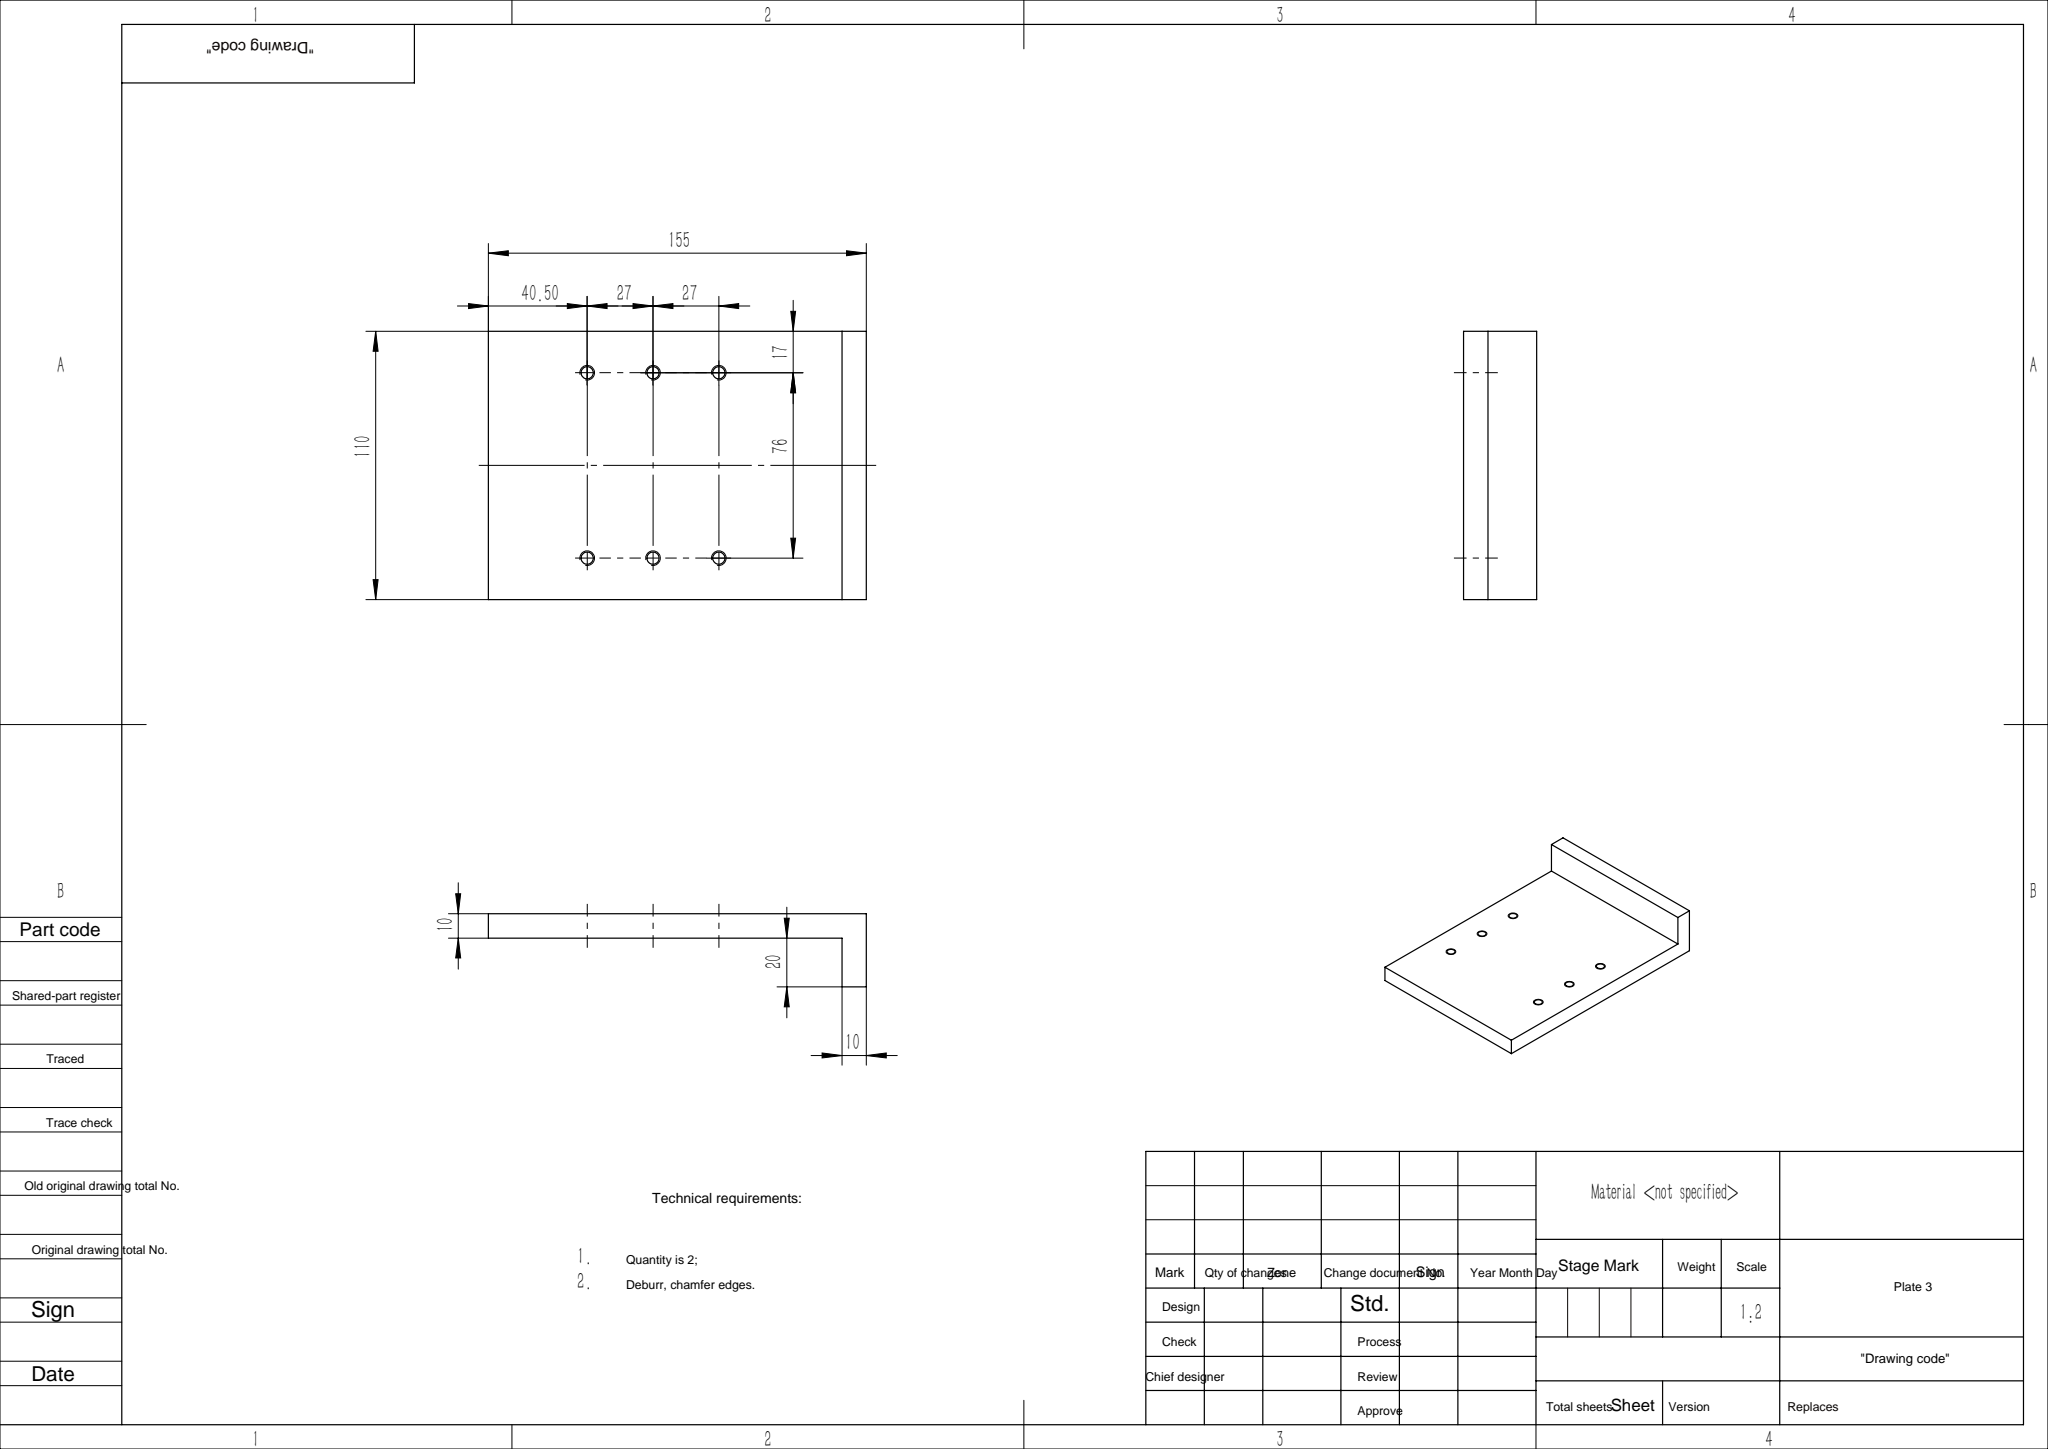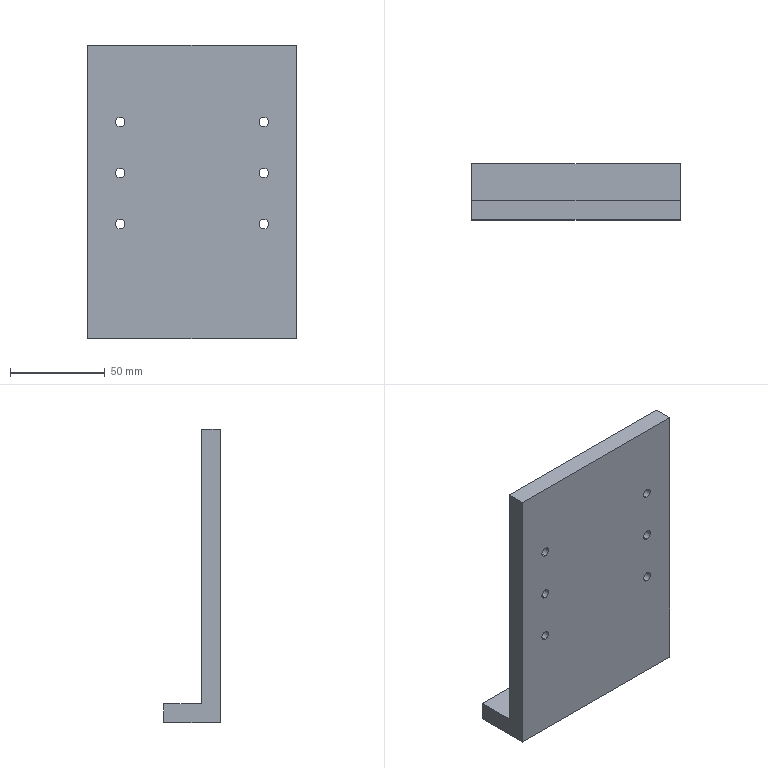Part | SolidWorks | features ICE 2, Extrusion 1, HoleWzd 1 | 1 solid | 20 faces | box 110 x 30 x 155 mm | volume 191322 mm3 | cylinder 12 | plane 8 | commonest cylinder face diameters 5 x12
STEP:
#1=CARTESIAN_POINT('',(-38.,0.,-29.5));
#2=VERTEX_POINT('',#1);
#3=CARTESIAN_POINT('',(-38.,0.,-24.5));
#4=VERTEX_POINT('',#3);
#5=CARTESIAN_POINT('',(-38.,0.,-27.));
#6=DIRECTION('',(0.,1.,0.));
#7=DIRECTION('',(0.,0.,1.));
#8=AXIS2_PLACEMENT_3D('',#5,#6,#7);
#9=CIRCLE('',#8,2.5);
#10=EDGE_CURVE('',#2,#4,#9,.T.);
#11=ORIENTED_EDGE('',*,*,#10,.F.);
#12=CARTESIAN_POINT('',(-38.,10.,-29.5));
#13=VERTEX_POINT('',#12);
#14=CARTESIAN_POINT('',(-38.,10.,-29.5));
#15=DIRECTION('',(0.,1.,0.));
#16=VECTOR('',#15,1000.);
#17=LINE('',#14,#16);
#18=EDGE_CURVE('',#2,#13,#17,.T.);
#19=ORIENTED_EDGE('',*,*,#18,.T.);
#20=CARTESIAN_POINT('',(-38.,10.,-24.5));
#21=VERTEX_POINT('',#20);
#22=CARTESIAN_POINT('',(-38.,10.,-27.));
#23=DIRECTION('',(0.,1.,0.));
#24=DIRECTION('',(0.,0.,1.));
#25=AXIS2_PLACEMENT_3D('',#22,#23,#24);
#26=CIRCLE('',#25,2.5);
#27=EDGE_CURVE('',#13,#21,#26,.T.);
#28=ORIENTED_EDGE('',*,*,#27,.T.);
#29=CARTESIAN_POINT('',(-38.,10.,-24.5));
#30=DIRECTION('',(0.,1.,0.));
#31=VECTOR('',#30,1000.);
#32=LINE('',#29,#31);
#33=EDGE_CURVE('',#4,#21,#32,.T.);
#34=ORIENTED_EDGE('',*,*,#33,.F.);
#35=EDGE_LOOP('',(#11,#19,#28,#34));
#36=FACE_OUTER_BOUND('',#35,.T.);
#37=CARTESIAN_POINT('',(-38.,10.,-27.));
#38=DIRECTION('',(0.,1.,0.));
#39=DIRECTION('',(0.,0.,1.));
#40=AXIS2_PLACEMENT_3D('',#37,#38,#39);
#41=CYLINDRICAL_SURFACE('',#40,2.5);
#42=ADVANCED_FACE('',(#36),#41,.F.);
#43=CARTESIAN_POINT('',(-38.,0.,-2.5));
#44=VERTEX_POINT('',#43);
#45=CARTESIAN_POINT('',(-38.,0.,2.5));
#46=VERTEX_POINT('',#45);
#47=CARTESIAN_POINT('',(-38.,0.,0.));
#48=DIRECTION('',(0.,1.,0.));
#49=DIRECTION('',(0.,0.,1.));
#50=AXIS2_PLACEMENT_3D('',#47,#48,#49);
#51=CIRCLE('',#50,2.5);
#52=EDGE_CURVE('',#44,#46,#51,.T.);
#53=ORIENTED_EDGE('',*,*,#52,.F.);
#54=CARTESIAN_POINT('',(-38.,10.,-2.5));
#55=VERTEX_POINT('',#54);
#56=CARTESIAN_POINT('',(-38.,10.,-2.5));
#57=DIRECTION('',(0.,1.,0.));
#58=VECTOR('',#57,1000.);
#59=LINE('',#56,#58);
#60=EDGE_CURVE('',#44,#55,#59,.T.);
#61=ORIENTED_EDGE('',*,*,#60,.T.);
#62=CARTESIAN_POINT('',(-38.,10.,2.5));
#63=VERTEX_POINT('',#62);
#64=CARTESIAN_POINT('',(-38.,10.,0.));
#65=DIRECTION('',(0.,1.,0.));
#66=DIRECTION('',(0.,0.,1.));
#67=AXIS2_PLACEMENT_3D('',#64,#65,#66);
#68=CIRCLE('',#67,2.5);
#69=EDGE_CURVE('',#55,#63,#68,.T.);
#70=ORIENTED_EDGE('',*,*,#69,.T.);
#71=CARTESIAN_POINT('',(-38.,10.,2.5));
#72=DIRECTION('',(0.,1.,0.));
#73=VECTOR('',#72,1000.);
#74=LINE('',#71,#73);
#75=EDGE_CURVE('',#46,#63,#74,.T.);
#76=ORIENTED_EDGE('',*,*,#75,.F.);
#77=EDGE_LOOP('',(#53,#61,#70,#76));
#78=FACE_OUTER_BOUND('',#77,.T.);
#79=CARTESIAN_POINT('',(-38.,10.,0.));
#80=DIRECTION('',(0.,1.,0.));
#81=DIRECTION('',(0.,0.,1.));
#82=AXIS2_PLACEMENT_3D('',#79,#80,#81);
#83=CYLINDRICAL_SURFACE('',#82,2.5);
#84=ADVANCED_FACE('',(#78),#83,.F.);
#85=CARTESIAN_POINT('',(38.,0.,-2.5));
#86=VERTEX_POINT('',#85);
#87=CARTESIAN_POINT('',(38.,0.,2.5));
#88=VERTEX_POINT('',#87);
#89=CARTESIAN_POINT('',(38.,0.,0.));
#90=DIRECTION('',(0.,1.,0.));
#91=DIRECTION('',(0.,0.,1.));
#92=AXIS2_PLACEMENT_3D('',#89,#90,#91);
#93=CIRCLE('',#92,2.5);
#94=EDGE_CURVE('',#86,#88,#93,.T.);
#95=ORIENTED_EDGE('',*,*,#94,.F.);
#96=CARTESIAN_POINT('',(38.,10.,-2.5));
#97=VERTEX_POINT('',#96);
#98=CARTESIAN_POINT('',(38.,10.,-2.5));
#99=DIRECTION('',(0.,1.,0.));
#100=VECTOR('',#99,1000.);
#101=LINE('',#98,#100);
#102=EDGE_CURVE('',#86,#97,#101,.T.);
#103=ORIENTED_EDGE('',*,*,#102,.T.);
#104=CARTESIAN_POINT('',(38.,10.,2.5));
#105=VERTEX_POINT('',#104);
#106=CARTESIAN_POINT('',(38.,10.,0.));
#107=DIRECTION('',(0.,1.,0.));
#108=DIRECTION('',(0.,0.,1.));
#109=AXIS2_PLACEMENT_3D('',#106,#107,#108);
#110=CIRCLE('',#109,2.5);
#111=EDGE_CURVE('',#97,#105,#110,.T.);
#112=ORIENTED_EDGE('',*,*,#111,.T.);
#113=CARTESIAN_POINT('',(38.,10.,2.5));
#114=DIRECTION('',(0.,1.,0.));
#115=VECTOR('',#114,1000.);
#116=LINE('',#113,#115);
#117=EDGE_CURVE('',#88,#105,#116,.T.);
#118=ORIENTED_EDGE('',*,*,#117,.F.);
#119=EDGE_LOOP('',(#95,#103,#112,#118));
#120=FACE_OUTER_BOUND('',#119,.T.);
#121=CARTESIAN_POINT('',(38.,10.,0.));
#122=DIRECTION('',(0.,1.,0.));
#123=DIRECTION('',(0.,0.,1.));
#124=AXIS2_PLACEMENT_3D('',#121,#122,#123);
#125=CYLINDRICAL_SURFACE('',#124,2.5);
#126=ADVANCED_FACE('',(#120),#125,.F.);
#127=CARTESIAN_POINT('',(-38.,0.,24.5));
#128=VERTEX_POINT('',#127);
#129=CARTESIAN_POINT('',(-38.,0.,29.5));
#130=VERTEX_POINT('',#129);
#131=CARTESIAN_POINT('',(-38.,0.,27.));
#132=DIRECTION('',(0.,1.,0.));
#133=DIRECTION('',(0.,0.,1.));
#134=AXIS2_PLACEMENT_3D('',#131,#132,#133);
#135=CIRCLE('',#134,2.5);
#136=EDGE_CURVE('',#128,#130,#135,.T.);
#137=ORIENTED_EDGE('',*,*,#136,.F.);
#138=CARTESIAN_POINT('',(-38.,10.,24.5));
#139=VERTEX_POINT('',#138);
#140=CARTESIAN_POINT('',(-38.,10.,24.5));
#141=DIRECTION('',(0.,1.,0.));
#142=VECTOR('',#141,1000.);
#143=LINE('',#140,#142);
#144=EDGE_CURVE('',#128,#139,#143,.T.);
#145=ORIENTED_EDGE('',*,*,#144,.T.);
#146=CARTESIAN_POINT('',(-38.,10.,29.5));
#147=VERTEX_POINT('',#146);
#148=CARTESIAN_POINT('',(-38.,10.,27.));
#149=DIRECTION('',(0.,1.,0.));
#150=DIRECTION('',(0.,0.,1.));
#151=AXIS2_PLACEMENT_3D('',#148,#149,#150);
#152=CIRCLE('',#151,2.5);
#153=EDGE_CURVE('',#139,#147,#152,.T.);
#154=ORIENTED_EDGE('',*,*,#153,.T.);
#155=CARTESIAN_POINT('',(-38.,10.,29.5));
#156=DIRECTION('',(0.,1.,0.));
#157=VECTOR('',#156,1000.);
#158=LINE('',#155,#157);
#159=EDGE_CURVE('',#130,#147,#158,.T.);
#160=ORIENTED_EDGE('',*,*,#159,.F.);
#161=EDGE_LOOP('',(#137,#145,#154,#160));
#162=FACE_OUTER_BOUND('',#161,.T.);
#163=CARTESIAN_POINT('',(-38.,10.,27.));
#164=DIRECTION('',(0.,1.,0.));
#165=DIRECTION('',(0.,0.,1.));
#166=AXIS2_PLACEMENT_3D('',#163,#164,#165);
#167=CYLINDRICAL_SURFACE('',#166,2.5);
#168=ADVANCED_FACE('',(#162),#167,.F.);
#169=CARTESIAN_POINT('',(38.,0.,24.5));
#170=VERTEX_POINT('',#169);
#171=CARTESIAN_POINT('',(38.,0.,29.5));
#172=VERTEX_POINT('',#171);
#173=CARTESIAN_POINT('',(38.,0.,27.));
#174=DIRECTION('',(0.,1.,0.));
#175=DIRECTION('',(0.,0.,1.));
#176=AXIS2_PLACEMENT_3D('',#173,#174,#175);
#177=CIRCLE('',#176,2.5);
#178=EDGE_CURVE('',#170,#172,#177,.T.);
#179=ORIENTED_EDGE('',*,*,#178,.F.);
#180=CARTESIAN_POINT('',(38.,10.,24.5));
#181=VERTEX_POINT('',#180);
#182=CARTESIAN_POINT('',(38.,10.,24.5));
#183=DIRECTION('',(0.,1.,0.));
#184=VECTOR('',#183,1000.);
#185=LINE('',#182,#184);
#186=EDGE_CURVE('',#170,#181,#185,.T.);
#187=ORIENTED_EDGE('',*,*,#186,.T.);
#188=CARTESIAN_POINT('',(38.,10.,29.5));
#189=VERTEX_POINT('',#188);
#190=CARTESIAN_POINT('',(38.,10.,27.));
#191=DIRECTION('',(0.,1.,0.));
#192=DIRECTION('',(0.,0.,1.));
#193=AXIS2_PLACEMENT_3D('',#190,#191,#192);
#194=CIRCLE('',#193,2.5);
#195=EDGE_CURVE('',#181,#189,#194,.T.);
#196=ORIENTED_EDGE('',*,*,#195,.T.);
#197=CARTESIAN_POINT('',(38.,10.,29.5));
#198=DIRECTION('',(0.,1.,0.));
#199=VECTOR('',#198,1000.);
#200=LINE('',#197,#199);
#201=EDGE_CURVE('',#172,#189,#200,.T.);
#202=ORIENTED_EDGE('',*,*,#201,.F.);
#203=EDGE_LOOP('',(#179,#187,#196,#202));
#204=FACE_OUTER_BOUND('',#203,.T.);
#205=CARTESIAN_POINT('',(38.,10.,27.));
#206=DIRECTION('',(0.,1.,0.));
#207=DIRECTION('',(0.,0.,1.));
#208=AXIS2_PLACEMENT_3D('',#205,#206,#207);
#209=CYLINDRICAL_SURFACE('',#208,2.5);
#210=ADVANCED_FACE('',(#204),#209,.F.);
#211=CARTESIAN_POINT('',(38.,0.,-29.5));
#212=VERTEX_POINT('',#211);
#213=CARTESIAN_POINT('',(38.,0.,-24.5));
#214=VERTEX_POINT('',#213);
#215=CARTESIAN_POINT('',(38.,0.,-27.));
#216=DIRECTION('',(0.,1.,0.));
#217=DIRECTION('',(0.,0.,1.));
#218=AXIS2_PLACEMENT_3D('',#215,#216,#217);
#219=CIRCLE('',#218,2.5);
#220=EDGE_CURVE('',#212,#214,#219,.T.);
#221=ORIENTED_EDGE('',*,*,#220,.F.);
#222=CARTESIAN_POINT('',(38.,10.,-29.5));
#223=VERTEX_POINT('',#222);
#224=CARTESIAN_POINT('',(38.,10.,-29.5));
#225=DIRECTION('',(0.,1.,0.));
#226=VECTOR('',#225,1000.);
#227=LINE('',#224,#226);
#228=EDGE_CURVE('',#212,#223,#227,.T.);
#229=ORIENTED_EDGE('',*,*,#228,.T.);
#230=CARTESIAN_POINT('',(38.,10.,-24.5));
#231=VERTEX_POINT('',#230);
#232=CARTESIAN_POINT('',(38.,10.,-27.));
#233=DIRECTION('',(0.,1.,0.));
#234=DIRECTION('',(0.,0.,1.));
#235=AXIS2_PLACEMENT_3D('',#232,#233,#234);
#236=CIRCLE('',#235,2.5);
#237=EDGE_CURVE('',#223,#231,#236,.T.);
#238=ORIENTED_EDGE('',*,*,#237,.T.);
#239=CARTESIAN_POINT('',(38.,10.,-24.5));
#240=DIRECTION('',(0.,1.,0.));
#241=VECTOR('',#240,1000.);
#242=LINE('',#239,#241);
#243=EDGE_CURVE('',#214,#231,#242,.T.);
#244=ORIENTED_EDGE('',*,*,#243,.F.);
#245=EDGE_LOOP('',(#221,#229,#238,#244));
#246=FACE_OUTER_BOUND('',#245,.T.);
#247=CARTESIAN_POINT('',(38.,10.,-27.));
#248=DIRECTION('',(0.,1.,0.));
#249=DIRECTION('',(0.,0.,1.));
#250=AXIS2_PLACEMENT_3D('',#247,#248,#249);
#251=CYLINDRICAL_SURFACE('',#250,2.5);
#252=ADVANCED_FACE('',(#246),#251,.F.);
#253=CARTESIAN_POINT('',(38.,10.,-27.));
#254=DIRECTION('',(0.,1.,0.));
#255=DIRECTION('',(0.,0.,1.));
#256=AXIS2_PLACEMENT_3D('',#253,#254,#255);
#257=CIRCLE('',#256,2.5);
#258=EDGE_CURVE('',#231,#223,#257,.T.);
#259=ORIENTED_EDGE('',*,*,#258,.F.);
#260=ORIENTED_EDGE('',*,*,#237,.F.);
#261=EDGE_LOOP('',(#259,#260));
#262=FACE_BOUND('',#261,.T.);
#263=CARTESIAN_POINT('',(38.,10.,27.));
#264=DIRECTION('',(0.,1.,0.));
#265=DIRECTION('',(0.,0.,1.));
#266=AXIS2_PLACEMENT_3D('',#263,#264,#265);
#267=CIRCLE('',#266,2.5);
#268=EDGE_CURVE('',#189,#181,#267,.T.);
#269=ORIENTED_EDGE('',*,*,#268,.F.);
#270=ORIENTED_EDGE('',*,*,#195,.F.);
#271=EDGE_LOOP('',(#269,#270));
#272=FACE_BOUND('',#271,.T.);
#273=CARTESIAN_POINT('',(-38.,10.,27.));
#274=DIRECTION('',(0.,1.,0.));
#275=DIRECTION('',(0.,0.,1.));
#276=AXIS2_PLACEMENT_3D('',#273,#274,#275);
#277=CIRCLE('',#276,2.5);
#278=EDGE_CURVE('',#147,#139,#277,.T.);
#279=ORIENTED_EDGE('',*,*,#278,.F.);
#280=ORIENTED_EDGE('',*,*,#153,.F.);
#281=EDGE_LOOP('',(#279,#280));
#282=FACE_BOUND('',#281,.T.);
#283=CARTESIAN_POINT('',(38.,10.,0.));
#284=DIRECTION('',(0.,1.,0.));
#285=DIRECTION('',(0.,0.,1.));
#286=AXIS2_PLACEMENT_3D('',#283,#284,#285);
#287=CIRCLE('',#286,2.5);
#288=EDGE_CURVE('',#105,#97,#287,.T.);
#289=ORIENTED_EDGE('',*,*,#288,.F.);
#290=ORIENTED_EDGE('',*,*,#111,.F.);
#291=EDGE_LOOP('',(#289,#290));
#292=FACE_BOUND('',#291,.T.);
#293=CARTESIAN_POINT('',(-38.,10.,0.));
#294=DIRECTION('',(0.,1.,0.));
#295=DIRECTION('',(0.,0.,1.));
#296=AXIS2_PLACEMENT_3D('',#293,#294,#295);
#297=CIRCLE('',#296,2.5);
#298=EDGE_CURVE('',#63,#55,#297,.T.);
#299=ORIENTED_EDGE('',*,*,#298,.F.);
#300=ORIENTED_EDGE('',*,*,#69,.F.);
#301=EDGE_LOOP('',(#299,#300));
#302=FACE_BOUND('',#301,.T.);
#303=CARTESIAN_POINT('',(-38.,10.,-27.));
#304=DIRECTION('',(0.,1.,0.));
#305=DIRECTION('',(0.,0.,1.));
#306=AXIS2_PLACEMENT_3D('',#303,#304,#305);
#307=CIRCLE('',#306,2.5);
#308=EDGE_CURVE('',#21,#13,#307,.T.);
#309=ORIENTED_EDGE('',*,*,#308,.F.);
#310=ORIENTED_EDGE('',*,*,#27,.F.);
#311=EDGE_LOOP('',(#309,#310));
#312=FACE_BOUND('',#311,.T.);
#313=CARTESIAN_POINT('',(-55.,10.,-77.5));
#314=VERTEX_POINT('',#313);
#315=CARTESIAN_POINT('',(55.,10.,-77.5));
#316=VERTEX_POINT('',#315);
#317=CARTESIAN_POINT('',(0.,10.,-77.5));
#318=DIRECTION('',(1.,0.,0.));
#319=VECTOR('',#318,1000.);
#320=LINE('',#317,#319);
#321=EDGE_CURVE('',#314,#316,#320,.T.);
#322=ORIENTED_EDGE('',*,*,#321,.F.);
#323=CARTESIAN_POINT('',(-55.,10.,67.5));
#324=VERTEX_POINT('',#323);
#325=CARTESIAN_POINT('',(-55.,10.,67.5));
#326=DIRECTION('',(0.,0.,1.));
#327=VECTOR('',#326,1000.);
#328=LINE('',#325,#327);
#329=EDGE_CURVE('',#314,#324,#328,.T.);
#330=ORIENTED_EDGE('',*,*,#329,.T.);
#331=CARTESIAN_POINT('',(55.,10.,67.5));
#332=VERTEX_POINT('',#331);
#333=CARTESIAN_POINT('',(-55.,10.,67.5));
#334=DIRECTION('',(1.,0.,0.));
#335=VECTOR('',#334,1000.);
#336=LINE('',#333,#335);
#337=EDGE_CURVE('',#324,#332,#336,.T.);
#338=ORIENTED_EDGE('',*,*,#337,.T.);
#339=CARTESIAN_POINT('',(55.,10.,67.5));
#340=DIRECTION('',(0.,0.,-1.));
#341=VECTOR('',#340,1000.);
#342=LINE('',#339,#341);
#343=EDGE_CURVE('',#332,#316,#342,.T.);
#344=ORIENTED_EDGE('',*,*,#343,.T.);
#345=EDGE_LOOP('',(#322,#330,#338,#344));
#346=FACE_OUTER_BOUND('',#345,.T.);
#347=CARTESIAN_POINT('',(0.,10.,0.));
#348=DIRECTION('',(0.,-1.,0.));
#349=DIRECTION('',(0.,0.,-1.));
#350=AXIS2_PLACEMENT_3D('',#347,#348,#349);
#351=PLANE('',#350);
#352=ADVANCED_FACE('',(#262,#272,#282,#292,#302,#312,#346),#351,.F.);
#353=CARTESIAN_POINT('',(55.,30.,-87.5));
#354=VERTEX_POINT('',#353);
#355=CARTESIAN_POINT('',(55.,0.,-87.5));
#356=VERTEX_POINT('',#355);
#357=CARTESIAN_POINT('',(55.,10.,-87.5));
#358=DIRECTION('',(0.,-1.,0.));
#359=VECTOR('',#358,1000.);
#360=LINE('',#357,#359);
#361=EDGE_CURVE('',#354,#356,#360,.T.);
#362=ORIENTED_EDGE('',*,*,#361,.F.);
#363=CARTESIAN_POINT('',(55.,30.,-77.5));
#364=VERTEX_POINT('',#363);
#365=CARTESIAN_POINT('',(55.,30.,-77.5));
#366=DIRECTION('',(0.,0.,-1.));
#367=VECTOR('',#366,1000.);
#368=LINE('',#365,#367);
#369=EDGE_CURVE('',#364,#354,#368,.T.);
#370=ORIENTED_EDGE('',*,*,#369,.F.);
#371=CARTESIAN_POINT('',(55.,30.,-77.5));
#372=DIRECTION('',(0.,-1.,0.));
#373=VECTOR('',#372,1000.);
#374=LINE('',#371,#373);
#375=EDGE_CURVE('',#364,#316,#374,.T.);
#376=ORIENTED_EDGE('',*,*,#375,.T.);
#377=ORIENTED_EDGE('',*,*,#343,.F.);
#378=CARTESIAN_POINT('',(55.,0.,67.5));
#379=VERTEX_POINT('',#378);
#380=CARTESIAN_POINT('',(55.,10.,67.5));
#381=DIRECTION('',(0.,-1.,0.));
#382=VECTOR('',#381,1000.);
#383=LINE('',#380,#382);
#384=EDGE_CURVE('',#332,#379,#383,.T.);
#385=ORIENTED_EDGE('',*,*,#384,.T.);
#386=CARTESIAN_POINT('',(55.,0.,67.5));
#387=DIRECTION('',(0.,0.,-1.));
#388=VECTOR('',#387,1000.);
#389=LINE('',#386,#388);
#390=EDGE_CURVE('',#379,#356,#389,.T.);
#391=ORIENTED_EDGE('',*,*,#390,.T.);
#392=EDGE_LOOP('',(#362,#370,#376,#377,#385,#391));
#393=FACE_OUTER_BOUND('',#392,.T.);
#394=CARTESIAN_POINT('',(55.,10.,67.5));
#395=DIRECTION('',(-1.,0.,0.));
#396=DIRECTION('',(0.,0.,1.));
#397=AXIS2_PLACEMENT_3D('',#394,#395,#396);
#398=PLANE('',#397);
#399=ADVANCED_FACE('',(#393),#398,.F.);
#400=CARTESIAN_POINT('',(-55.,0.,-87.5));
#401=VERTEX_POINT('',#400);
#402=CARTESIAN_POINT('',(-55.,0.,67.5));
#403=VERTEX_POINT('',#402);
#404=CARTESIAN_POINT('',(-55.,0.,67.5));
#405=DIRECTION('',(0.,0.,1.));
#406=VECTOR('',#405,1000.);
#407=LINE('',#404,#406);
#408=EDGE_CURVE('',#401,#403,#407,.T.);
#409=ORIENTED_EDGE('',*,*,#408,.T.);
#410=CARTESIAN_POINT('',(-55.,10.,67.5));
#411=DIRECTION('',(0.,-1.,0.));
#412=VECTOR('',#411,1000.);
#413=LINE('',#410,#412);
#414=EDGE_CURVE('',#324,#403,#413,.T.);
#415=ORIENTED_EDGE('',*,*,#414,.F.);
#416=ORIENTED_EDGE('',*,*,#329,.F.);
#417=CARTESIAN_POINT('',(-55.,30.,-77.5));
#418=VERTEX_POINT('',#417);
#419=CARTESIAN_POINT('',(-55.,30.,-77.5));
#420=DIRECTION('',(0.,1.,0.));
#421=VECTOR('',#420,1000.);
#422=LINE('',#419,#421);
#423=EDGE_CURVE('',#314,#418,#422,.T.);
#424=ORIENTED_EDGE('',*,*,#423,.T.);
#425=CARTESIAN_POINT('',(-55.,30.,-87.5));
#426=VERTEX_POINT('',#425);
#427=CARTESIAN_POINT('',(-55.,30.,-77.5));
#428=DIRECTION('',(0.,0.,-1.));
#429=VECTOR('',#428,1000.);
#430=LINE('',#427,#429);
#431=EDGE_CURVE('',#418,#426,#430,.T.);
#432=ORIENTED_EDGE('',*,*,#431,.T.);
#433=CARTESIAN_POINT('',(-55.,10.,-87.5));
#434=DIRECTION('',(0.,-1.,0.));
#435=VECTOR('',#434,1000.);
#436=LINE('',#433,#435);
#437=EDGE_CURVE('',#426,#401,#436,.T.);
#438=ORIENTED_EDGE('',*,*,#437,.T.);
#439=EDGE_LOOP('',(#409,#415,#416,#424,#432,#438));
#440=FACE_OUTER_BOUND('',#439,.T.);
#441=CARTESIAN_POINT('',(-55.,10.,67.5));
#442=DIRECTION('',(1.,0.,0.));
#443=DIRECTION('',(0.,0.,-1.));
#444=AXIS2_PLACEMENT_3D('',#441,#442,#443);
#445=PLANE('',#444);
#446=ADVANCED_FACE('',(#440),#445,.F.);
#447=CARTESIAN_POINT('',(-55.,0.,67.5));
#448=DIRECTION('',(1.,0.,0.));
#449=VECTOR('',#448,1000.);
#450=LINE('',#447,#449);
#451=EDGE_CURVE('',#403,#379,#450,.T.);
#452=ORIENTED_EDGE('',*,*,#451,.T.);
#453=ORIENTED_EDGE('',*,*,#384,.F.);
#454=ORIENTED_EDGE('',*,*,#337,.F.);
#455=ORIENTED_EDGE('',*,*,#414,.T.);
#456=EDGE_LOOP('',(#452,#453,#454,#455));
#457=FACE_OUTER_BOUND('',#456,.T.);
#458=CARTESIAN_POINT('',(-55.,10.,67.5));
#459=DIRECTION('',(0.,0.,-1.));
#460=DIRECTION('',(-1.,0.,0.));
#461=AXIS2_PLACEMENT_3D('',#458,#459,#460);
#462=PLANE('',#461);
#463=ADVANCED_FACE('',(#457),#462,.F.);
#464=CARTESIAN_POINT('',(-55.,0.,-87.5));
#465=DIRECTION('',(1.,0.,0.));
#466=VECTOR('',#465,1000.);
#467=LINE('',#464,#466);
#468=EDGE_CURVE('',#401,#356,#467,.T.);
#469=ORIENTED_EDGE('',*,*,#468,.T.);
#470=ORIENTED_EDGE('',*,*,#390,.F.);
#471=ORIENTED_EDGE('',*,*,#451,.F.);
#472=ORIENTED_EDGE('',*,*,#408,.F.);
#473=EDGE_LOOP('',(#469,#470,#471,#472));
#474=FACE_OUTER_BOUND('',#473,.T.);
#475=CARTESIAN_POINT('',(38.,0.,-27.));
#476=DIRECTION('',(0.,1.,0.));
#477=DIRECTION('',(0.,0.,1.));
#478=AXIS2_PLACEMENT_3D('',#475,#476,#477);
#479=CIRCLE('',#478,2.5);
#480=EDGE_CURVE('',#214,#212,#479,.T.);
#481=ORIENTED_EDGE('',*,*,#480,.T.);
#482=ORIENTED_EDGE('',*,*,#220,.T.);
#483=EDGE_LOOP('',(#481,#482));
#484=FACE_BOUND('',#483,.T.);
#485=CARTESIAN_POINT('',(38.,0.,27.));
#486=DIRECTION('',(0.,1.,0.));
#487=DIRECTION('',(0.,0.,1.));
#488=AXIS2_PLACEMENT_3D('',#485,#486,#487);
#489=CIRCLE('',#488,2.5);
#490=EDGE_CURVE('',#172,#170,#489,.T.);
#491=ORIENTED_EDGE('',*,*,#490,.T.);
#492=ORIENTED_EDGE('',*,*,#178,.T.);
#493=EDGE_LOOP('',(#491,#492));
#494=FACE_BOUND('',#493,.T.);
#495=CARTESIAN_POINT('',(-38.,0.,27.));
#496=DIRECTION('',(0.,1.,0.));
#497=DIRECTION('',(0.,0.,1.));
#498=AXIS2_PLACEMENT_3D('',#495,#496,#497);
#499=CIRCLE('',#498,2.5);
#500=EDGE_CURVE('',#130,#128,#499,.T.);
#501=ORIENTED_EDGE('',*,*,#500,.T.);
#502=ORIENTED_EDGE('',*,*,#136,.T.);
#503=EDGE_LOOP('',(#501,#502));
#504=FACE_BOUND('',#503,.T.);
#505=CARTESIAN_POINT('',(38.,0.,0.));
#506=DIRECTION('',(0.,1.,0.));
#507=DIRECTION('',(0.,0.,1.));
#508=AXIS2_PLACEMENT_3D('',#505,#506,#507);
#509=CIRCLE('',#508,2.5);
#510=EDGE_CURVE('',#88,#86,#509,.T.);
#511=ORIENTED_EDGE('',*,*,#510,.T.);
#512=ORIENTED_EDGE('',*,*,#94,.T.);
#513=EDGE_LOOP('',(#511,#512));
#514=FACE_BOUND('',#513,.T.);
#515=CARTESIAN_POINT('',(-38.,0.,0.));
#516=DIRECTION('',(0.,1.,0.));
#517=DIRECTION('',(0.,0.,1.));
#518=AXIS2_PLACEMENT_3D('',#515,#516,#517);
#519=CIRCLE('',#518,2.5);
#520=EDGE_CURVE('',#46,#44,#519,.T.);
#521=ORIENTED_EDGE('',*,*,#520,.T.);
#522=ORIENTED_EDGE('',*,*,#52,.T.);
#523=EDGE_LOOP('',(#521,#522));
#524=FACE_BOUND('',#523,.T.);
#525=CARTESIAN_POINT('',(-38.,0.,-27.));
#526=DIRECTION('',(0.,1.,0.));
#527=DIRECTION('',(0.,0.,1.));
#528=AXIS2_PLACEMENT_3D('',#525,#526,#527);
#529=CIRCLE('',#528,2.5);
#530=EDGE_CURVE('',#4,#2,#529,.T.);
#531=ORIENTED_EDGE('',*,*,#530,.T.);
#532=ORIENTED_EDGE('',*,*,#10,.T.);
#533=EDGE_LOOP('',(#531,#532));
#534=FACE_BOUND('',#533,.T.);
#535=CARTESIAN_POINT('',(0.,0.,0.));
#536=DIRECTION('',(0.,-1.,0.));
#537=DIRECTION('',(0.,0.,-1.));
#538=AXIS2_PLACEMENT_3D('',#535,#536,#537);
#539=PLANE('',#538);
#540=ADVANCED_FACE('',(#474,#484,#494,#504,#514,#524,#534),#539,.T.);
#541=ORIENTED_EDGE('',*,*,#228,.F.);
#542=ORIENTED_EDGE('',*,*,#480,.F.);
#543=ORIENTED_EDGE('',*,*,#243,.T.);
#544=ORIENTED_EDGE('',*,*,#258,.T.);
#545=EDGE_LOOP('',(#541,#542,#543,#544));
#546=FACE_OUTER_BOUND('',#545,.T.);
#547=CARTESIAN_POINT('',(38.,10.,-27.));
#548=DIRECTION('',(0.,1.,0.));
#549=DIRECTION('',(0.,0.,1.));
#550=AXIS2_PLACEMENT_3D('',#547,#548,#549);
#551=CYLINDRICAL_SURFACE('',#550,2.5);
#552=ADVANCED_FACE('',(#546),#551,.F.);
#553=ORIENTED_EDGE('',*,*,#186,.F.);
#554=ORIENTED_EDGE('',*,*,#490,.F.);
#555=ORIENTED_EDGE('',*,*,#201,.T.);
#556=ORIENTED_EDGE('',*,*,#268,.T.);
#557=EDGE_LOOP('',(#553,#554,#555,#556));
#558=FACE_OUTER_BOUND('',#557,.T.);
#559=CARTESIAN_POINT('',(38.,10.,27.));
#560=DIRECTION('',(0.,1.,0.));
#561=DIRECTION('',(0.,0.,1.));
#562=AXIS2_PLACEMENT_3D('',#559,#560,#561);
#563=CYLINDRICAL_SURFACE('',#562,2.5);
#564=ADVANCED_FACE('',(#558),#563,.F.);
#565=ORIENTED_EDGE('',*,*,#144,.F.);
#566=ORIENTED_EDGE('',*,*,#500,.F.);
#567=ORIENTED_EDGE('',*,*,#159,.T.);
#568=ORIENTED_EDGE('',*,*,#278,.T.);
#569=EDGE_LOOP('',(#565,#566,#567,#568));
#570=FACE_OUTER_BOUND('',#569,.T.);
#571=CARTESIAN_POINT('',(-38.,10.,27.));
#572=DIRECTION('',(0.,1.,0.));
#573=DIRECTION('',(0.,0.,1.));
#574=AXIS2_PLACEMENT_3D('',#571,#572,#573);
#575=CYLINDRICAL_SURFACE('',#574,2.5);
#576=ADVANCED_FACE('',(#570),#575,.F.);
#577=ORIENTED_EDGE('',*,*,#102,.F.);
#578=ORIENTED_EDGE('',*,*,#510,.F.);
#579=ORIENTED_EDGE('',*,*,#117,.T.);
#580=ORIENTED_EDGE('',*,*,#288,.T.);
#581=EDGE_LOOP('',(#577,#578,#579,#580));
#582=FACE_OUTER_BOUND('',#581,.T.);
#583=CARTESIAN_POINT('',(38.,10.,0.));
#584=DIRECTION('',(0.,1.,0.));
#585=DIRECTION('',(0.,0.,1.));
#586=AXIS2_PLACEMENT_3D('',#583,#584,#585);
#587=CYLINDRICAL_SURFACE('',#586,2.5);
#588=ADVANCED_FACE('',(#582),#587,.F.);
#589=ORIENTED_EDGE('',*,*,#60,.F.);
#590=ORIENTED_EDGE('',*,*,#520,.F.);
#591=ORIENTED_EDGE('',*,*,#75,.T.);
#592=ORIENTED_EDGE('',*,*,#298,.T.);
#593=EDGE_LOOP('',(#589,#590,#591,#592));
#594=FACE_OUTER_BOUND('',#593,.T.);
#595=CARTESIAN_POINT('',(-38.,10.,0.));
#596=DIRECTION('',(0.,1.,0.));
#597=DIRECTION('',(0.,0.,1.));
#598=AXIS2_PLACEMENT_3D('',#595,#596,#597);
#599=CYLINDRICAL_SURFACE('',#598,2.5);
#600=ADVANCED_FACE('',(#594),#599,.F.);
#601=ORIENTED_EDGE('',*,*,#18,.F.);
#602=ORIENTED_EDGE('',*,*,#530,.F.);
#603=ORIENTED_EDGE('',*,*,#33,.T.);
#604=ORIENTED_EDGE('',*,*,#308,.T.);
#605=EDGE_LOOP('',(#601,#602,#603,#604));
#606=FACE_OUTER_BOUND('',#605,.T.);
#607=CARTESIAN_POINT('',(-38.,10.,-27.));
#608=DIRECTION('',(0.,1.,0.));
#609=DIRECTION('',(0.,0.,1.));
#610=AXIS2_PLACEMENT_3D('',#607,#608,#609);
#611=CYLINDRICAL_SURFACE('',#610,2.5);
#612=ADVANCED_FACE('',(#606),#611,.F.);
#613=ORIENTED_EDGE('',*,*,#468,.F.);
#614=ORIENTED_EDGE('',*,*,#437,.F.);
#615=CARTESIAN_POINT('',(55.,30.,-87.5));
#616=DIRECTION('',(1.,0.,0.));
#617=VECTOR('',#616,1000.);
#618=LINE('',#615,#617);
#619=EDGE_CURVE('',#426,#354,#618,.T.);
#620=ORIENTED_EDGE('',*,*,#619,.T.);
#621=ORIENTED_EDGE('',*,*,#361,.T.);
#622=EDGE_LOOP('',(#613,#614,#620,#621));
#623=FACE_OUTER_BOUND('',#622,.T.);
#624=CARTESIAN_POINT('',(-55.,10.,-87.5));
#625=DIRECTION('',(0.,0.,-1.));
#626=DIRECTION('',(-1.,0.,0.));
#627=AXIS2_PLACEMENT_3D('',#624,#625,#626);
#628=PLANE('',#627);
#629=ADVANCED_FACE('',(#623),#628,.T.);
#630=ORIENTED_EDGE('',*,*,#423,.F.);
#631=ORIENTED_EDGE('',*,*,#321,.T.);
#632=ORIENTED_EDGE('',*,*,#375,.F.);
#633=CARTESIAN_POINT('',(55.,30.,-77.5));
#634=DIRECTION('',(1.,0.,0.));
#635=VECTOR('',#634,1000.);
#636=LINE('',#633,#635);
#637=EDGE_CURVE('',#418,#364,#636,.T.);
#638=ORIENTED_EDGE('',*,*,#637,.F.);
#639=EDGE_LOOP('',(#630,#631,#632,#638));
#640=FACE_OUTER_BOUND('',#639,.T.);
#641=CARTESIAN_POINT('',(0.,0.,-77.5));
#642=DIRECTION('',(0.,0.,-1.));
#643=DIRECTION('',(-1.,0.,0.));
#644=AXIS2_PLACEMENT_3D('',#641,#642,#643);
#645=PLANE('',#644);
#646=ADVANCED_FACE('',(#640),#645,.F.);
#647=ORIENTED_EDGE('',*,*,#619,.F.);
#648=ORIENTED_EDGE('',*,*,#431,.F.);
#649=ORIENTED_EDGE('',*,*,#637,.T.);
#650=ORIENTED_EDGE('',*,*,#369,.T.);
#651=EDGE_LOOP('',(#647,#648,#649,#650));
#652=FACE_OUTER_BOUND('',#651,.T.);
#653=CARTESIAN_POINT('',(55.,30.,-77.5));
#654=DIRECTION('',(0.,1.,0.));
#655=DIRECTION('',(0.,0.,1.));
#656=AXIS2_PLACEMENT_3D('',#653,#654,#655);
#657=PLANE('',#656);
#658=ADVANCED_FACE('',(#652),#657,.T.);
#659=CLOSED_SHELL('',(#42,#84,#126,#168,#210,#252,#352,#399,#446,#463,#540,#552,#564,#576,#588,#600,#612,#629,#646,#658));
#660=MANIFOLD_SOLID_BREP('',#659);
#661=CARTESIAN_POINT('',(0.,0.,0.));
#662=DIRECTION('',(0.,0.,1.));
#663=DIRECTION('',(1.,0.,0.));
#664=AXIS2_PLACEMENT_3D('',#661,#662,#663);
#665=(LENGTH_UNIT()NAMED_UNIT(*)SI_UNIT(.MILLI.,.METRE.));
#666=UNCERTAINTY_MEASURE_WITH_UNIT(LENGTH_MEASURE(0.00001),#665,'','');
#667=(NAMED_UNIT(*)PLANE_ANGLE_UNIT()SI_UNIT($,.RADIAN.));
#668=(NAMED_UNIT(*)SI_UNIT($,.STERADIAN.)SOLID_ANGLE_UNIT());
#669=(GEOMETRIC_REPRESENTATION_CONTEXT(3)GLOBAL_UNCERTAINTY_ASSIGNED_CONTEXT((#666))GLOBAL_UNIT_ASSIGNED_CONTEXT((#665,#667,#668))REPRESENTATION_CONTEXT('',''));
#670=ADVANCED_BREP_SHAPE_REPRESENTATION('',(#660,#664),#669);